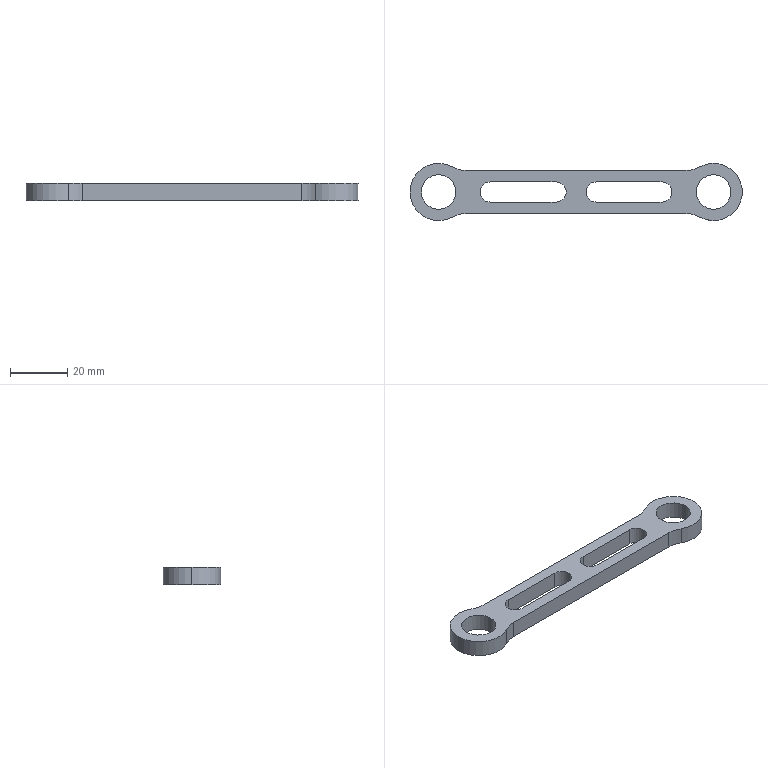Part | SolidWorks | features Extrusion 1, Fillet 1 | 1 solid | 25 faces | box 116 x 20 x 6 mm | volume 7064 mm3 | cylinder 17 | plane 8 | commonest cylinder face diameters 20 x7 7 x6 12 x4
STEP:
#1=CARTESIAN_POINT('',(55.,3.5,6.));
#2=VERTEX_POINT('',#1);
#3=CARTESIAN_POINT('',(51.5,0.,6.));
#4=VERTEX_POINT('',#3);
#5=CARTESIAN_POINT('',(55.,0.,6.));
#6=DIRECTION('',(0.,0.,1.));
#7=DIRECTION('',(1.,0.,0.));
#8=AXIS2_PLACEMENT_3D('',#5,#6,#7);
#9=CIRCLE('',#8,3.5);
#10=EDGE_CURVE('',#2,#4,#9,.T.);
#11=ORIENTED_EDGE('',*,*,#10,.T.);
#12=CARTESIAN_POINT('',(51.5,0.,0.));
#13=VERTEX_POINT('',#12);
#14=CARTESIAN_POINT('',(51.5,0.,6.));
#15=DIRECTION('',(0.,0.,-1.));
#16=VECTOR('',#15,1000.);
#17=LINE('',#14,#16);
#18=EDGE_CURVE('',#4,#13,#17,.T.);
#19=ORIENTED_EDGE('',*,*,#18,.T.);
#20=CARTESIAN_POINT('',(55.,3.5,0.));
#21=VERTEX_POINT('',#20);
#22=CARTESIAN_POINT('',(55.,0.,0.));
#23=DIRECTION('',(0.,0.,1.));
#24=DIRECTION('',(1.,0.,0.));
#25=AXIS2_PLACEMENT_3D('',#22,#23,#24);
#26=CIRCLE('',#25,3.5);
#27=EDGE_CURVE('',#21,#13,#26,.T.);
#28=ORIENTED_EDGE('',*,*,#27,.F.);
#29=CARTESIAN_POINT('',(55.,3.5,6.));
#30=DIRECTION('',(0.,0.,-1.));
#31=VECTOR('',#30,1000.);
#32=LINE('',#29,#31);
#33=EDGE_CURVE('',#2,#21,#32,.T.);
#34=ORIENTED_EDGE('',*,*,#33,.F.);
#35=EDGE_LOOP('',(#11,#19,#28,#34));
#36=FACE_OUTER_BOUND('',#35,.T.);
#37=CARTESIAN_POINT('',(55.,0.,6.));
#38=DIRECTION('',(0.,0.,-1.));
#39=DIRECTION('',(-1.,0.,0.));
#40=AXIS2_PLACEMENT_3D('',#37,#38,#39);
#41=CYLINDRICAL_SURFACE('',#40,3.5);
#42=ADVANCED_FACE('',(#36),#41,.F.);
#43=CARTESIAN_POINT('',(18.,3.5,6.));
#44=VERTEX_POINT('',#43);
#45=CARTESIAN_POINT('',(14.5,0.,6.));
#46=VERTEX_POINT('',#45);
#47=CARTESIAN_POINT('',(18.,0.,6.));
#48=DIRECTION('',(0.,0.,1.));
#49=DIRECTION('',(1.,0.,0.));
#50=AXIS2_PLACEMENT_3D('',#47,#48,#49);
#51=CIRCLE('',#50,3.5);
#52=EDGE_CURVE('',#44,#46,#51,.T.);
#53=ORIENTED_EDGE('',*,*,#52,.T.);
#54=CARTESIAN_POINT('',(14.5,0.,0.));
#55=VERTEX_POINT('',#54);
#56=CARTESIAN_POINT('',(14.5,0.,6.));
#57=DIRECTION('',(0.,0.,-1.));
#58=VECTOR('',#57,1000.);
#59=LINE('',#56,#58);
#60=EDGE_CURVE('',#46,#55,#59,.T.);
#61=ORIENTED_EDGE('',*,*,#60,.T.);
#62=CARTESIAN_POINT('',(18.,3.5,0.));
#63=VERTEX_POINT('',#62);
#64=CARTESIAN_POINT('',(18.,0.,0.));
#65=DIRECTION('',(0.,0.,1.));
#66=DIRECTION('',(1.,0.,0.));
#67=AXIS2_PLACEMENT_3D('',#64,#65,#66);
#68=CIRCLE('',#67,3.5);
#69=EDGE_CURVE('',#63,#55,#68,.T.);
#70=ORIENTED_EDGE('',*,*,#69,.F.);
#71=CARTESIAN_POINT('',(18.,3.5,6.));
#72=DIRECTION('',(0.,0.,-1.));
#73=VECTOR('',#72,1000.);
#74=LINE('',#71,#73);
#75=EDGE_CURVE('',#44,#63,#74,.T.);
#76=ORIENTED_EDGE('',*,*,#75,.F.);
#77=EDGE_LOOP('',(#53,#61,#70,#76));
#78=FACE_OUTER_BOUND('',#77,.T.);
#79=CARTESIAN_POINT('',(18.,0.,6.));
#80=DIRECTION('',(0.,0.,-1.));
#81=DIRECTION('',(-1.,0.,0.));
#82=AXIS2_PLACEMENT_3D('',#79,#80,#81);
#83=CYLINDRICAL_SURFACE('',#82,3.5);
#84=ADVANCED_FACE('',(#78),#83,.F.);
#85=CARTESIAN_POINT('',(90.,0.,6.));
#86=VERTEX_POINT('',#85);
#87=CARTESIAN_POINT('',(102.,0.,6.));
#88=VERTEX_POINT('',#87);
#89=CARTESIAN_POINT('',(96.,0.,6.));
#90=DIRECTION('',(0.,0.,1.));
#91=DIRECTION('',(1.,0.,0.));
#92=AXIS2_PLACEMENT_3D('',#89,#90,#91);
#93=CIRCLE('',#92,6.);
#94=EDGE_CURVE('',#86,#88,#93,.T.);
#95=ORIENTED_EDGE('',*,*,#94,.T.);
#96=CARTESIAN_POINT('',(102.,0.,0.));
#97=VERTEX_POINT('',#96);
#98=CARTESIAN_POINT('',(102.,0.,6.));
#99=DIRECTION('',(0.,0.,-1.));
#100=VECTOR('',#99,1000.);
#101=LINE('',#98,#100);
#102=EDGE_CURVE('',#88,#97,#101,.T.);
#103=ORIENTED_EDGE('',*,*,#102,.T.);
#104=CARTESIAN_POINT('',(90.,0.,0.));
#105=VERTEX_POINT('',#104);
#106=CARTESIAN_POINT('',(96.,0.,0.));
#107=DIRECTION('',(0.,0.,1.));
#108=DIRECTION('',(1.,0.,0.));
#109=AXIS2_PLACEMENT_3D('',#106,#107,#108);
#110=CIRCLE('',#109,6.);
#111=EDGE_CURVE('',#105,#97,#110,.T.);
#112=ORIENTED_EDGE('',*,*,#111,.F.);
#113=CARTESIAN_POINT('',(90.,0.,6.));
#114=DIRECTION('',(0.,0.,-1.));
#115=VECTOR('',#114,1000.);
#116=LINE('',#113,#115);
#117=EDGE_CURVE('',#86,#105,#116,.T.);
#118=ORIENTED_EDGE('',*,*,#117,.F.);
#119=EDGE_LOOP('',(#95,#103,#112,#118));
#120=FACE_OUTER_BOUND('',#119,.T.);
#121=CARTESIAN_POINT('',(96.,0.,6.));
#122=DIRECTION('',(0.,0.,-1.));
#123=DIRECTION('',(-1.,0.,0.));
#124=AXIS2_PLACEMENT_3D('',#121,#122,#123);
#125=CYLINDRICAL_SURFACE('',#124,6.);
#126=ADVANCED_FACE('',(#120),#125,.F.);
#127=CARTESIAN_POINT('',(-6.,0.,6.));
#128=VERTEX_POINT('',#127);
#129=CARTESIAN_POINT('',(6.,0.,6.));
#130=VERTEX_POINT('',#129);
#131=CARTESIAN_POINT('',(0.,0.,6.));
#132=DIRECTION('',(0.,0.,1.));
#133=DIRECTION('',(1.,0.,0.));
#134=AXIS2_PLACEMENT_3D('',#131,#132,#133);
#135=CIRCLE('',#134,6.);
#136=EDGE_CURVE('',#128,#130,#135,.T.);
#137=ORIENTED_EDGE('',*,*,#136,.T.);
#138=CARTESIAN_POINT('',(6.,0.,0.));
#139=VERTEX_POINT('',#138);
#140=CARTESIAN_POINT('',(6.,0.,6.));
#141=DIRECTION('',(0.,0.,-1.));
#142=VECTOR('',#141,1000.);
#143=LINE('',#140,#142);
#144=EDGE_CURVE('',#130,#139,#143,.T.);
#145=ORIENTED_EDGE('',*,*,#144,.T.);
#146=CARTESIAN_POINT('',(-6.,0.,0.));
#147=VERTEX_POINT('',#146);
#148=CARTESIAN_POINT('',(0.,0.,0.));
#149=DIRECTION('',(0.,0.,1.));
#150=DIRECTION('',(1.,0.,0.));
#151=AXIS2_PLACEMENT_3D('',#148,#149,#150);
#152=CIRCLE('',#151,6.);
#153=EDGE_CURVE('',#147,#139,#152,.T.);
#154=ORIENTED_EDGE('',*,*,#153,.F.);
#155=CARTESIAN_POINT('',(-6.,0.,6.));
#156=DIRECTION('',(0.,0.,-1.));
#157=VECTOR('',#156,1000.);
#158=LINE('',#155,#157);
#159=EDGE_CURVE('',#128,#147,#158,.T.);
#160=ORIENTED_EDGE('',*,*,#159,.F.);
#161=EDGE_LOOP('',(#137,#145,#154,#160));
#162=FACE_OUTER_BOUND('',#161,.T.);
#163=CARTESIAN_POINT('',(0.,0.,6.));
#164=DIRECTION('',(0.,0.,-1.));
#165=DIRECTION('',(-1.,0.,0.));
#166=AXIS2_PLACEMENT_3D('',#163,#164,#165);
#167=CYLINDRICAL_SURFACE('',#166,6.);
#168=ADVANCED_FACE('',(#162),#167,.F.);
#169=CARTESIAN_POINT('',(-10.,0.,6.));
#170=VERTEX_POINT('',#169);
#171=CARTESIAN_POINT('',(4.841,-8.75,6.));
#172=VERTEX_POINT('',#171);
#173=CARTESIAN_POINT('',(0.,0.,6.));
#174=DIRECTION('',(0.,0.,1.));
#175=DIRECTION('',(1.,0.,0.));
#176=AXIS2_PLACEMENT_3D('',#173,#174,#175);
#177=CIRCLE('',#176,10.);
#178=EDGE_CURVE('',#170,#172,#177,.T.);
#179=ORIENTED_EDGE('',*,*,#178,.F.);
#180=CARTESIAN_POINT('',(-10.,0.,0.));
#181=VERTEX_POINT('',#180);
#182=CARTESIAN_POINT('',(-10.,0.,6.));
#183=DIRECTION('',(0.,0.,-1.));
#184=VECTOR('',#183,1000.);
#185=LINE('',#182,#184);
#186=EDGE_CURVE('',#170,#181,#185,.T.);
#187=ORIENTED_EDGE('',*,*,#186,.T.);
#188=CARTESIAN_POINT('',(4.841,-8.75,0.));
#189=VERTEX_POINT('',#188);
#190=CARTESIAN_POINT('',(0.,0.,0.));
#191=DIRECTION('',(0.,0.,1.));
#192=DIRECTION('',(1.,0.,0.));
#193=AXIS2_PLACEMENT_3D('',#190,#191,#192);
#194=CIRCLE('',#193,10.);
#195=EDGE_CURVE('',#181,#189,#194,.T.);
#196=ORIENTED_EDGE('',*,*,#195,.T.);
#197=CARTESIAN_POINT('',(4.841,-8.75,6.));
#198=DIRECTION('',(0.,0.,1.));
#199=VECTOR('',#198,1000.);
#200=LINE('',#197,#199);
#201=EDGE_CURVE('',#189,#172,#200,.T.);
#202=ORIENTED_EDGE('',*,*,#201,.T.);
#203=EDGE_LOOP('',(#179,#187,#196,#202));
#204=FACE_OUTER_BOUND('',#203,.T.);
#205=CARTESIAN_POINT('',(0.,0.,6.));
#206=DIRECTION('',(0.,0.,-1.));
#207=DIRECTION('',(-1.,0.,0.));
#208=AXIS2_PLACEMENT_3D('',#205,#206,#207);
#209=CYLINDRICAL_SURFACE('',#208,10.);
#210=ADVANCED_FACE('',(#204),#209,.T.);
#211=ORIENTED_EDGE('',*,*,#136,.F.);
#212=CARTESIAN_POINT('',(0.,0.,6.));
#213=DIRECTION('',(0.,0.,1.));
#214=DIRECTION('',(1.,0.,0.));
#215=AXIS2_PLACEMENT_3D('',#212,#213,#214);
#216=CIRCLE('',#215,6.);
#217=EDGE_CURVE('',#130,#128,#216,.T.);
#218=ORIENTED_EDGE('',*,*,#217,.F.);
#219=EDGE_LOOP('',(#211,#218));
#220=FACE_BOUND('',#219,.T.);
#221=CARTESIAN_POINT('',(86.318,7.5,6.));
#222=VERTEX_POINT('',#221);
#223=CARTESIAN_POINT('',(9.682,7.5,6.));
#224=VERTEX_POINT('',#223);
#225=CARTESIAN_POINT('',(6.614,7.5,6.));
#226=DIRECTION('',(-1.,0.,0.));
#227=VECTOR('',#226,1000.);
#228=LINE('',#225,#227);
#229=EDGE_CURVE('',#222,#224,#228,.T.);
#230=ORIENTED_EDGE('',*,*,#229,.T.);
#231=CARTESIAN_POINT('',(4.841,8.75,6.));
#232=VERTEX_POINT('',#231);
#233=CARTESIAN_POINT('',(9.682,17.5,6.));
#234=DIRECTION('',(0.,0.,-1.));
#235=DIRECTION('',(1.,0.,0.));
#236=AXIS2_PLACEMENT_3D('',#233,#234,#235);
#237=CIRCLE('',#236,10.);
#238=EDGE_CURVE('',#224,#232,#237,.T.);
#239=ORIENTED_EDGE('',*,*,#238,.T.);
#240=CARTESIAN_POINT('',(0.,0.,6.));
#241=DIRECTION('',(0.,0.,1.));
#242=DIRECTION('',(1.,0.,0.));
#243=AXIS2_PLACEMENT_3D('',#240,#241,#242);
#244=CIRCLE('',#243,10.);
#245=EDGE_CURVE('',#232,#170,#244,.T.);
#246=ORIENTED_EDGE('',*,*,#245,.T.);
#247=ORIENTED_EDGE('',*,*,#178,.T.);
#248=CARTESIAN_POINT('',(9.682,-7.5,6.));
#249=VERTEX_POINT('',#248);
#250=CARTESIAN_POINT('',(9.682,-17.5,6.));
#251=DIRECTION('',(0.,0.,-1.));
#252=DIRECTION('',(1.,0.,0.));
#253=AXIS2_PLACEMENT_3D('',#250,#251,#252);
#254=CIRCLE('',#253,10.);
#255=EDGE_CURVE('',#172,#249,#254,.T.);
#256=ORIENTED_EDGE('',*,*,#255,.T.);
#257=CARTESIAN_POINT('',(86.318,-7.5,6.));
#258=VERTEX_POINT('',#257);
#259=CARTESIAN_POINT('',(6.614,-7.5,6.));
#260=DIRECTION('',(1.,0.,0.));
#261=VECTOR('',#260,1000.);
#262=LINE('',#259,#261);
#263=EDGE_CURVE('',#249,#258,#262,.T.);
#264=ORIENTED_EDGE('',*,*,#263,.T.);
#265=CARTESIAN_POINT('',(91.159,-8.75,6.));
#266=VERTEX_POINT('',#265);
#267=CARTESIAN_POINT('',(86.318,-17.5,6.));
#268=DIRECTION('',(0.,0.,-1.));
#269=DIRECTION('',(1.,0.,0.));
#270=AXIS2_PLACEMENT_3D('',#267,#268,#269);
#271=CIRCLE('',#270,10.);
#272=EDGE_CURVE('',#258,#266,#271,.T.);
#273=ORIENTED_EDGE('',*,*,#272,.T.);
#274=CARTESIAN_POINT('',(91.159,8.75,6.));
#275=VERTEX_POINT('',#274);
#276=CARTESIAN_POINT('',(96.,0.,6.));
#277=DIRECTION('',(0.,0.,1.));
#278=DIRECTION('',(1.,0.,0.));
#279=AXIS2_PLACEMENT_3D('',#276,#277,#278);
#280=CIRCLE('',#279,10.);
#281=EDGE_CURVE('',#266,#275,#280,.T.);
#282=ORIENTED_EDGE('',*,*,#281,.T.);
#283=CARTESIAN_POINT('',(86.318,17.5,6.));
#284=DIRECTION('',(0.,0.,-1.));
#285=DIRECTION('',(1.,0.,0.));
#286=AXIS2_PLACEMENT_3D('',#283,#284,#285);
#287=CIRCLE('',#286,10.);
#288=EDGE_CURVE('',#275,#222,#287,.T.);
#289=ORIENTED_EDGE('',*,*,#288,.T.);
#290=EDGE_LOOP('',(#230,#239,#246,#247,#256,#264,#273,#282,#289));
#291=FACE_OUTER_BOUND('',#290,.T.);
#292=ORIENTED_EDGE('',*,*,#94,.F.);
#293=CARTESIAN_POINT('',(96.,0.,6.));
#294=DIRECTION('',(0.,0.,1.));
#295=DIRECTION('',(1.,0.,0.));
#296=AXIS2_PLACEMENT_3D('',#293,#294,#295);
#297=CIRCLE('',#296,6.);
#298=EDGE_CURVE('',#88,#86,#297,.T.);
#299=ORIENTED_EDGE('',*,*,#298,.F.);
#300=EDGE_LOOP('',(#292,#299));
#301=FACE_BOUND('',#300,.T.);
#302=CARTESIAN_POINT('',(18.,-3.5,6.));
#303=VERTEX_POINT('',#302);
#304=CARTESIAN_POINT('',(41.,-3.5,6.));
#305=VERTEX_POINT('',#304);
#306=CARTESIAN_POINT('',(18.,-3.5,6.));
#307=DIRECTION('',(1.,0.,0.));
#308=VECTOR('',#307,1000.);
#309=LINE('',#306,#308);
#310=EDGE_CURVE('',#303,#305,#309,.T.);
#311=ORIENTED_EDGE('',*,*,#310,.F.);
#312=CARTESIAN_POINT('',(18.,0.,6.));
#313=DIRECTION('',(0.,0.,1.));
#314=DIRECTION('',(1.,0.,0.));
#315=AXIS2_PLACEMENT_3D('',#312,#313,#314);
#316=CIRCLE('',#315,3.5);
#317=EDGE_CURVE('',#46,#303,#316,.T.);
#318=ORIENTED_EDGE('',*,*,#317,.F.);
#319=ORIENTED_EDGE('',*,*,#52,.F.);
#320=CARTESIAN_POINT('',(41.,3.5,6.));
#321=VERTEX_POINT('',#320);
#322=CARTESIAN_POINT('',(18.,3.5,6.));
#323=DIRECTION('',(-1.,0.,0.));
#324=VECTOR('',#323,1000.);
#325=LINE('',#322,#324);
#326=EDGE_CURVE('',#321,#44,#325,.T.);
#327=ORIENTED_EDGE('',*,*,#326,.F.);
#328=CARTESIAN_POINT('',(41.,0.,6.));
#329=DIRECTION('',(0.,0.,1.));
#330=DIRECTION('',(1.,0.,0.));
#331=AXIS2_PLACEMENT_3D('',#328,#329,#330);
#332=CIRCLE('',#331,3.5);
#333=EDGE_CURVE('',#305,#321,#332,.T.);
#334=ORIENTED_EDGE('',*,*,#333,.F.);
#335=EDGE_LOOP('',(#311,#318,#319,#327,#334));
#336=FACE_BOUND('',#335,.T.);
#337=CARTESIAN_POINT('',(78.,3.5,6.));
#338=VERTEX_POINT('',#337);
#339=CARTESIAN_POINT('',(78.,3.5,6.));
#340=DIRECTION('',(-1.,0.,0.));
#341=VECTOR('',#340,1000.);
#342=LINE('',#339,#341);
#343=EDGE_CURVE('',#338,#2,#342,.T.);
#344=ORIENTED_EDGE('',*,*,#343,.F.);
#345=CARTESIAN_POINT('',(78.,-3.5,6.));
#346=VERTEX_POINT('',#345);
#347=CARTESIAN_POINT('',(78.,0.,6.));
#348=DIRECTION('',(0.,0.,1.));
#349=DIRECTION('',(1.,0.,0.));
#350=AXIS2_PLACEMENT_3D('',#347,#348,#349);
#351=CIRCLE('',#350,3.5);
#352=EDGE_CURVE('',#346,#338,#351,.T.);
#353=ORIENTED_EDGE('',*,*,#352,.F.);
#354=CARTESIAN_POINT('',(55.,-3.5,6.));
#355=VERTEX_POINT('',#354);
#356=CARTESIAN_POINT('',(78.,-3.5,6.));
#357=DIRECTION('',(1.,0.,0.));
#358=VECTOR('',#357,1000.);
#359=LINE('',#356,#358);
#360=EDGE_CURVE('',#355,#346,#359,.T.);
#361=ORIENTED_EDGE('',*,*,#360,.F.);
#362=CARTESIAN_POINT('',(55.,0.,6.));
#363=DIRECTION('',(0.,0.,1.));
#364=DIRECTION('',(1.,0.,0.));
#365=AXIS2_PLACEMENT_3D('',#362,#363,#364);
#366=CIRCLE('',#365,3.5);
#367=EDGE_CURVE('',#4,#355,#366,.T.);
#368=ORIENTED_EDGE('',*,*,#367,.F.);
#369=ORIENTED_EDGE('',*,*,#10,.F.);
#370=EDGE_LOOP('',(#344,#353,#361,#368,#369));
#371=FACE_BOUND('',#370,.T.);
#372=CARTESIAN_POINT('',(0.,0.,6.));
#373=DIRECTION('',(0.,0.,1.));
#374=DIRECTION('',(1.,0.,0.));
#375=AXIS2_PLACEMENT_3D('',#372,#373,#374);
#376=PLANE('',#375);
#377=ADVANCED_FACE('',(#220,#291,#301,#336,#371),#376,.T.);
#378=ORIENTED_EDGE('',*,*,#69,.T.);
#379=CARTESIAN_POINT('',(18.,-3.5,0.));
#380=VERTEX_POINT('',#379);
#381=CARTESIAN_POINT('',(18.,0.,0.));
#382=DIRECTION('',(0.,0.,1.));
#383=DIRECTION('',(1.,0.,0.));
#384=AXIS2_PLACEMENT_3D('',#381,#382,#383);
#385=CIRCLE('',#384,3.5);
#386=EDGE_CURVE('',#55,#380,#385,.T.);
#387=ORIENTED_EDGE('',*,*,#386,.T.);
#388=CARTESIAN_POINT('',(41.,-3.5,0.));
#389=VERTEX_POINT('',#388);
#390=CARTESIAN_POINT('',(18.,-3.5,0.));
#391=DIRECTION('',(1.,0.,0.));
#392=VECTOR('',#391,1000.);
#393=LINE('',#390,#392);
#394=EDGE_CURVE('',#380,#389,#393,.T.);
#395=ORIENTED_EDGE('',*,*,#394,.T.);
#396=CARTESIAN_POINT('',(41.,3.5,0.));
#397=VERTEX_POINT('',#396);
#398=CARTESIAN_POINT('',(41.,0.,0.));
#399=DIRECTION('',(0.,0.,1.));
#400=DIRECTION('',(1.,0.,0.));
#401=AXIS2_PLACEMENT_3D('',#398,#399,#400);
#402=CIRCLE('',#401,3.5);
#403=EDGE_CURVE('',#389,#397,#402,.T.);
#404=ORIENTED_EDGE('',*,*,#403,.T.);
#405=CARTESIAN_POINT('',(18.,3.5,0.));
#406=DIRECTION('',(-1.,0.,0.));
#407=VECTOR('',#406,1000.);
#408=LINE('',#405,#407);
#409=EDGE_CURVE('',#397,#63,#408,.T.);
#410=ORIENTED_EDGE('',*,*,#409,.T.);
#411=EDGE_LOOP('',(#378,#387,#395,#404,#410));
#412=FACE_BOUND('',#411,.T.);
#413=CARTESIAN_POINT('',(4.841,8.75,0.));
#414=VERTEX_POINT('',#413);
#415=CARTESIAN_POINT('',(0.,0.,0.));
#416=DIRECTION('',(0.,0.,1.));
#417=DIRECTION('',(1.,0.,0.));
#418=AXIS2_PLACEMENT_3D('',#415,#416,#417);
#419=CIRCLE('',#418,10.);
#420=EDGE_CURVE('',#414,#181,#419,.T.);
#421=ORIENTED_EDGE('',*,*,#420,.F.);
#422=CARTESIAN_POINT('',(9.682,7.5,0.));
#423=VERTEX_POINT('',#422);
#424=CARTESIAN_POINT('',(9.682,17.5,0.));
#425=DIRECTION('',(0.,0.,1.));
#426=DIRECTION('',(1.,0.,0.));
#427=AXIS2_PLACEMENT_3D('',#424,#425,#426);
#428=CIRCLE('',#427,10.);
#429=EDGE_CURVE('',#414,#423,#428,.T.);
#430=ORIENTED_EDGE('',*,*,#429,.T.);
#431=CARTESIAN_POINT('',(86.318,7.5,0.));
#432=VERTEX_POINT('',#431);
#433=CARTESIAN_POINT('',(6.614,7.5,0.));
#434=DIRECTION('',(-1.,0.,0.));
#435=VECTOR('',#434,1000.);
#436=LINE('',#433,#435);
#437=EDGE_CURVE('',#432,#423,#436,.T.);
#438=ORIENTED_EDGE('',*,*,#437,.F.);
#439=CARTESIAN_POINT('',(91.159,8.75,0.));
#440=VERTEX_POINT('',#439);
#441=CARTESIAN_POINT('',(86.318,17.5,0.));
#442=DIRECTION('',(0.,0.,1.));
#443=DIRECTION('',(1.,0.,0.));
#444=AXIS2_PLACEMENT_3D('',#441,#442,#443);
#445=CIRCLE('',#444,10.);
#446=EDGE_CURVE('',#432,#440,#445,.T.);
#447=ORIENTED_EDGE('',*,*,#446,.T.);
#448=CARTESIAN_POINT('',(91.159,-8.75,0.));
#449=VERTEX_POINT('',#448);
#450=CARTESIAN_POINT('',(96.,0.,0.));
#451=DIRECTION('',(0.,0.,1.));
#452=DIRECTION('',(1.,0.,0.));
#453=AXIS2_PLACEMENT_3D('',#450,#451,#452);
#454=CIRCLE('',#453,10.);
#455=EDGE_CURVE('',#449,#440,#454,.T.);
#456=ORIENTED_EDGE('',*,*,#455,.F.);
#457=CARTESIAN_POINT('',(86.318,-7.5,0.));
#458=VERTEX_POINT('',#457);
#459=CARTESIAN_POINT('',(86.318,-17.5,0.));
#460=DIRECTION('',(0.,0.,1.));
#461=DIRECTION('',(1.,0.,0.));
#462=AXIS2_PLACEMENT_3D('',#459,#460,#461);
#463=CIRCLE('',#462,10.);
#464=EDGE_CURVE('',#449,#458,#463,.T.);
#465=ORIENTED_EDGE('',*,*,#464,.T.);
#466=CARTESIAN_POINT('',(9.682,-7.5,0.));
#467=VERTEX_POINT('',#466);
#468=CARTESIAN_POINT('',(6.614,-7.5,0.));
#469=DIRECTION('',(1.,0.,0.));
#470=VECTOR('',#469,1000.);
#471=LINE('',#468,#470);
#472=EDGE_CURVE('',#467,#458,#471,.T.);
#473=ORIENTED_EDGE('',*,*,#472,.F.);
#474=CARTESIAN_POINT('',(9.682,-17.5,0.));
#475=DIRECTION('',(0.,0.,1.));
#476=DIRECTION('',(1.,0.,0.));
#477=AXIS2_PLACEMENT_3D('',#474,#475,#476);
#478=CIRCLE('',#477,10.);
#479=EDGE_CURVE('',#467,#189,#478,.T.);
#480=ORIENTED_EDGE('',*,*,#479,.T.);
#481=ORIENTED_EDGE('',*,*,#195,.F.);
#482=EDGE_LOOP('',(#421,#430,#438,#447,#456,#465,#473,#480,#481));
#483=FACE_OUTER_BOUND('',#482,.T.);
#484=ORIENTED_EDGE('',*,*,#153,.T.);
#485=CARTESIAN_POINT('',(0.,0.,0.));
#486=DIRECTION('',(0.,0.,1.));
#487=DIRECTION('',(1.,0.,0.));
#488=AXIS2_PLACEMENT_3D('',#485,#486,#487);
#489=CIRCLE('',#488,6.);
#490=EDGE_CURVE('',#139,#147,#489,.T.);
#491=ORIENTED_EDGE('',*,*,#490,.T.);
#492=EDGE_LOOP('',(#484,#491));
#493=FACE_BOUND('',#492,.T.);
#494=ORIENTED_EDGE('',*,*,#111,.T.);
#495=CARTESIAN_POINT('',(96.,0.,0.));
#496=DIRECTION('',(0.,0.,1.));
#497=DIRECTION('',(1.,0.,0.));
#498=AXIS2_PLACEMENT_3D('',#495,#496,#497);
#499=CIRCLE('',#498,6.);
#500=EDGE_CURVE('',#97,#105,#499,.T.);
#501=ORIENTED_EDGE('',*,*,#500,.T.);
#502=EDGE_LOOP('',(#494,#501));
#503=FACE_BOUND('',#502,.T.);
#504=CARTESIAN_POINT('',(78.,-3.5,0.));
#505=VERTEX_POINT('',#504);
#506=CARTESIAN_POINT('',(78.,3.5,0.));
#507=VERTEX_POINT('',#506);
#508=CARTESIAN_POINT('',(78.,0.,0.));
#509=DIRECTION('',(0.,0.,1.));
#510=DIRECTION('',(1.,0.,0.));
#511=AXIS2_PLACEMENT_3D('',#508,#509,#510);
#512=CIRCLE('',#511,3.5);
#513=EDGE_CURVE('',#505,#507,#512,.T.);
#514=ORIENTED_EDGE('',*,*,#513,.T.);
#515=CARTESIAN_POINT('',(78.,3.5,0.));
#516=DIRECTION('',(-1.,0.,0.));
#517=VECTOR('',#516,1000.);
#518=LINE('',#515,#517);
#519=EDGE_CURVE('',#507,#21,#518,.T.);
#520=ORIENTED_EDGE('',*,*,#519,.T.);
#521=ORIENTED_EDGE('',*,*,#27,.T.);
#522=CARTESIAN_POINT('',(55.,-3.5,0.));
#523=VERTEX_POINT('',#522);
#524=CARTESIAN_POINT('',(55.,0.,0.));
#525=DIRECTION('',(0.,0.,1.));
#526=DIRECTION('',(1.,0.,0.));
#527=AXIS2_PLACEMENT_3D('',#524,#525,#526);
#528=CIRCLE('',#527,3.5);
#529=EDGE_CURVE('',#13,#523,#528,.T.);
#530=ORIENTED_EDGE('',*,*,#529,.T.);
#531=CARTESIAN_POINT('',(78.,-3.5,0.));
#532=DIRECTION('',(1.,0.,0.));
#533=VECTOR('',#532,1000.);
#534=LINE('',#531,#533);
#535=EDGE_CURVE('',#523,#505,#534,.T.);
#536=ORIENTED_EDGE('',*,*,#535,.T.);
#537=EDGE_LOOP('',(#514,#520,#521,#530,#536));
#538=FACE_BOUND('',#537,.T.);
#539=CARTESIAN_POINT('',(0.,0.,0.));
#540=DIRECTION('',(0.,0.,1.));
#541=DIRECTION('',(1.,0.,0.));
#542=AXIS2_PLACEMENT_3D('',#539,#540,#541);
#543=PLANE('',#542);
#544=ADVANCED_FACE('',(#412,#483,#493,#503,#538),#543,.F.);
#545=ORIENTED_EDGE('',*,*,#186,.F.);
#546=ORIENTED_EDGE('',*,*,#245,.F.);
#547=CARTESIAN_POINT('',(4.841,8.75,6.));
#548=DIRECTION('',(0.,0.,-1.));
#549=VECTOR('',#548,1000.);
#550=LINE('',#547,#549);
#551=EDGE_CURVE('',#232,#414,#550,.T.);
#552=ORIENTED_EDGE('',*,*,#551,.T.);
#553=ORIENTED_EDGE('',*,*,#420,.T.);
#554=EDGE_LOOP('',(#545,#546,#552,#553));
#555=FACE_OUTER_BOUND('',#554,.T.);
#556=CARTESIAN_POINT('',(0.,0.,6.));
#557=DIRECTION('',(0.,0.,-1.));
#558=DIRECTION('',(-1.,0.,0.));
#559=AXIS2_PLACEMENT_3D('',#556,#557,#558);
#560=CYLINDRICAL_SURFACE('',#559,10.);
#561=ADVANCED_FACE('',(#555),#560,.T.);
#562=ORIENTED_EDGE('',*,*,#263,.F.);
#563=CARTESIAN_POINT('',(9.682,-7.5,0.));
#564=DIRECTION('',(0.,0.,-1.));
#565=VECTOR('',#564,1000.);
#566=LINE('',#563,#565);
#567=EDGE_CURVE('',#249,#467,#566,.T.);
#568=ORIENTED_EDGE('',*,*,#567,.T.);
#569=ORIENTED_EDGE('',*,*,#472,.T.);
#570=CARTESIAN_POINT('',(86.318,-7.5,6.));
#571=DIRECTION('',(0.,0.,1.));
#572=VECTOR('',#571,1000.);
#573=LINE('',#570,#572);
#574=EDGE_CURVE('',#458,#258,#573,.T.);
#575=ORIENTED_EDGE('',*,*,#574,.T.);
#576=EDGE_LOOP('',(#562,#568,#569,#575));
#577=FACE_OUTER_BOUND('',#576,.T.);
#578=CARTESIAN_POINT('',(6.614,-7.5,6.));
#579=DIRECTION('',(0.,1.,0.));
#580=DIRECTION('',(0.,0.,1.));
#581=AXIS2_PLACEMENT_3D('',#578,#579,#580);
#582=PLANE('',#581);
#583=ADVANCED_FACE('',(#577),#582,.F.);
#584=ORIENTED_EDGE('',*,*,#281,.F.);
#585=CARTESIAN_POINT('',(91.159,-8.75,6.));
#586=DIRECTION('',(0.,0.,-1.));
#587=VECTOR('',#586,1000.);
#588=LINE('',#585,#587);
#589=EDGE_CURVE('',#266,#449,#588,.T.);
#590=ORIENTED_EDGE('',*,*,#589,.T.);
#591=ORIENTED_EDGE('',*,*,#455,.T.);
#592=CARTESIAN_POINT('',(91.159,8.75,6.));
#593=DIRECTION('',(0.,0.,1.));
#594=VECTOR('',#593,1000.);
#595=LINE('',#592,#594);
#596=EDGE_CURVE('',#440,#275,#595,.T.);
#597=ORIENTED_EDGE('',*,*,#596,.T.);
#598=EDGE_LOOP('',(#584,#590,#591,#597));
#599=FACE_OUTER_BOUND('',#598,.T.);
#600=CARTESIAN_POINT('',(96.,0.,6.));
#601=DIRECTION('',(0.,0.,-1.));
#602=DIRECTION('',(-1.,0.,0.));
#603=AXIS2_PLACEMENT_3D('',#600,#601,#602);
#604=CYLINDRICAL_SURFACE('',#603,10.);
#605=ADVANCED_FACE('',(#599),#604,.T.);
#606=ORIENTED_EDGE('',*,*,#229,.F.);
#607=CARTESIAN_POINT('',(86.318,7.5,0.));
#608=DIRECTION('',(0.,0.,-1.));
#609=VECTOR('',#608,1000.);
#610=LINE('',#607,#609);
#611=EDGE_CURVE('',#222,#432,#610,.T.);
#612=ORIENTED_EDGE('',*,*,#611,.T.);
#613=ORIENTED_EDGE('',*,*,#437,.T.);
#614=CARTESIAN_POINT('',(9.682,7.5,6.));
#615=DIRECTION('',(0.,0.,1.));
#616=VECTOR('',#615,1000.);
#617=LINE('',#614,#616);
#618=EDGE_CURVE('',#423,#224,#617,.T.);
#619=ORIENTED_EDGE('',*,*,#618,.T.);
#620=EDGE_LOOP('',(#606,#612,#613,#619));
#621=FACE_OUTER_BOUND('',#620,.T.);
#622=CARTESIAN_POINT('',(6.614,7.5,6.));
#623=DIRECTION('',(0.,-1.,0.));
#624=DIRECTION('',(0.,0.,-1.));
#625=AXIS2_PLACEMENT_3D('',#622,#623,#624);
#626=PLANE('',#625);
#627=ADVANCED_FACE('',(#621),#626,.F.);
#628=ORIENTED_EDGE('',*,*,#144,.F.);
#629=ORIENTED_EDGE('',*,*,#217,.T.);
#630=ORIENTED_EDGE('',*,*,#159,.T.);
#631=ORIENTED_EDGE('',*,*,#490,.F.);
#632=EDGE_LOOP('',(#628,#629,#630,#631));
#633=FACE_OUTER_BOUND('',#632,.T.);
#634=CARTESIAN_POINT('',(0.,0.,6.));
#635=DIRECTION('',(0.,0.,-1.));
#636=DIRECTION('',(-1.,0.,0.));
#637=AXIS2_PLACEMENT_3D('',#634,#635,#636);
#638=CYLINDRICAL_SURFACE('',#637,6.);
#639=ADVANCED_FACE('',(#633),#638,.F.);
#640=ORIENTED_EDGE('',*,*,#102,.F.);
#641=ORIENTED_EDGE('',*,*,#298,.T.);
#642=ORIENTED_EDGE('',*,*,#117,.T.);
#643=ORIENTED_EDGE('',*,*,#500,.F.);
#644=EDGE_LOOP('',(#640,#641,#642,#643));
#645=FACE_OUTER_BOUND('',#644,.T.);
#646=CARTESIAN_POINT('',(96.,0.,6.));
#647=DIRECTION('',(0.,0.,-1.));
#648=DIRECTION('',(-1.,0.,0.));
#649=AXIS2_PLACEMENT_3D('',#646,#647,#648);
#650=CYLINDRICAL_SURFACE('',#649,6.);
#651=ADVANCED_FACE('',(#645),#650,.F.);
#652=ORIENTED_EDGE('',*,*,#60,.F.);
#653=ORIENTED_EDGE('',*,*,#317,.T.);
#654=CARTESIAN_POINT('',(18.,-3.5,6.));
#655=DIRECTION('',(0.,0.,-1.));
#656=VECTOR('',#655,1000.);
#657=LINE('',#654,#656);
#658=EDGE_CURVE('',#303,#380,#657,.T.);
#659=ORIENTED_EDGE('',*,*,#658,.T.);
#660=ORIENTED_EDGE('',*,*,#386,.F.);
#661=EDGE_LOOP('',(#652,#653,#659,#660));
#662=FACE_OUTER_BOUND('',#661,.T.);
#663=CARTESIAN_POINT('',(18.,0.,6.));
#664=DIRECTION('',(0.,0.,-1.));
#665=DIRECTION('',(-1.,0.,0.));
#666=AXIS2_PLACEMENT_3D('',#663,#664,#665);
#667=CYLINDRICAL_SURFACE('',#666,3.5);
#668=ADVANCED_FACE('',(#662),#667,.F.);
#669=ORIENTED_EDGE('',*,*,#394,.F.);
#670=ORIENTED_EDGE('',*,*,#658,.F.);
#671=ORIENTED_EDGE('',*,*,#310,.T.);
#672=CARTESIAN_POINT('',(41.,-3.5,6.));
#673=DIRECTION('',(0.,0.,-1.));
#674=VECTOR('',#673,1000.);
#675=LINE('',#672,#674);
#676=EDGE_CURVE('',#305,#389,#675,.T.);
#677=ORIENTED_EDGE('',*,*,#676,.T.);
#678=EDGE_LOOP('',(#669,#670,#671,#677));
#679=FACE_OUTER_BOUND('',#678,.T.);
#680=CARTESIAN_POINT('',(18.,-3.5,6.));
#681=DIRECTION('',(0.,1.,0.));
#682=DIRECTION('',(0.,0.,1.));
#683=AXIS2_PLACEMENT_3D('',#680,#681,#682);
#684=PLANE('',#683);
#685=ADVANCED_FACE('',(#679),#684,.T.);
#686=ORIENTED_EDGE('',*,*,#403,.F.);
#687=ORIENTED_EDGE('',*,*,#676,.F.);
#688=ORIENTED_EDGE('',*,*,#333,.T.);
#689=CARTESIAN_POINT('',(41.,3.5,6.));
#690=DIRECTION('',(0.,0.,-1.));
#691=VECTOR('',#690,1000.);
#692=LINE('',#689,#691);
#693=EDGE_CURVE('',#321,#397,#692,.T.);
#694=ORIENTED_EDGE('',*,*,#693,.T.);
#695=EDGE_LOOP('',(#686,#687,#688,#694));
#696=FACE_OUTER_BOUND('',#695,.T.);
#697=CARTESIAN_POINT('',(41.,0.,6.));
#698=DIRECTION('',(0.,0.,-1.));
#699=DIRECTION('',(-1.,0.,0.));
#700=AXIS2_PLACEMENT_3D('',#697,#698,#699);
#701=CYLINDRICAL_SURFACE('',#700,3.5);
#702=ADVANCED_FACE('',(#696),#701,.F.);
#703=ORIENTED_EDGE('',*,*,#409,.F.);
#704=ORIENTED_EDGE('',*,*,#693,.F.);
#705=ORIENTED_EDGE('',*,*,#326,.T.);
#706=ORIENTED_EDGE('',*,*,#75,.T.);
#707=EDGE_LOOP('',(#703,#704,#705,#706));
#708=FACE_OUTER_BOUND('',#707,.T.);
#709=CARTESIAN_POINT('',(18.,3.5,6.));
#710=DIRECTION('',(0.,-1.,0.));
#711=DIRECTION('',(0.,0.,-1.));
#712=AXIS2_PLACEMENT_3D('',#709,#710,#711);
#713=PLANE('',#712);
#714=ADVANCED_FACE('',(#708),#713,.T.);
#715=ORIENTED_EDGE('',*,*,#513,.F.);
#716=CARTESIAN_POINT('',(78.,-3.5,6.));
#717=DIRECTION('',(0.,0.,-1.));
#718=VECTOR('',#717,1000.);
#719=LINE('',#716,#718);
#720=EDGE_CURVE('',#346,#505,#719,.T.);
#721=ORIENTED_EDGE('',*,*,#720,.F.);
#722=ORIENTED_EDGE('',*,*,#352,.T.);
#723=CARTESIAN_POINT('',(78.,3.5,6.));
#724=DIRECTION('',(0.,0.,-1.));
#725=VECTOR('',#724,1000.);
#726=LINE('',#723,#725);
#727=EDGE_CURVE('',#338,#507,#726,.T.);
#728=ORIENTED_EDGE('',*,*,#727,.T.);
#729=EDGE_LOOP('',(#715,#721,#722,#728));
#730=FACE_OUTER_BOUND('',#729,.T.);
#731=CARTESIAN_POINT('',(78.,0.,6.));
#732=DIRECTION('',(0.,0.,-1.));
#733=DIRECTION('',(-1.,0.,0.));
#734=AXIS2_PLACEMENT_3D('',#731,#732,#733);
#735=CYLINDRICAL_SURFACE('',#734,3.5);
#736=ADVANCED_FACE('',(#730),#735,.F.);
#737=ORIENTED_EDGE('',*,*,#519,.F.);
#738=ORIENTED_EDGE('',*,*,#727,.F.);
#739=ORIENTED_EDGE('',*,*,#343,.T.);
#740=ORIENTED_EDGE('',*,*,#33,.T.);
#741=EDGE_LOOP('',(#737,#738,#739,#740));
#742=FACE_OUTER_BOUND('',#741,.T.);
#743=CARTESIAN_POINT('',(78.,3.5,6.));
#744=DIRECTION('',(0.,-1.,0.));
#745=DIRECTION('',(0.,0.,-1.));
#746=AXIS2_PLACEMENT_3D('',#743,#744,#745);
#747=PLANE('',#746);
#748=ADVANCED_FACE('',(#742),#747,.T.);
#749=ORIENTED_EDGE('',*,*,#18,.F.);
#750=ORIENTED_EDGE('',*,*,#367,.T.);
#751=CARTESIAN_POINT('',(55.,-3.5,6.));
#752=DIRECTION('',(0.,0.,-1.));
#753=VECTOR('',#752,1000.);
#754=LINE('',#751,#753);
#755=EDGE_CURVE('',#355,#523,#754,.T.);
#756=ORIENTED_EDGE('',*,*,#755,.T.);
#757=ORIENTED_EDGE('',*,*,#529,.F.);
#758=EDGE_LOOP('',(#749,#750,#756,#757));
#759=FACE_OUTER_BOUND('',#758,.T.);
#760=CARTESIAN_POINT('',(55.,0.,6.));
#761=DIRECTION('',(0.,0.,-1.));
#762=DIRECTION('',(-1.,0.,0.));
#763=AXIS2_PLACEMENT_3D('',#760,#761,#762);
#764=CYLINDRICAL_SURFACE('',#763,3.5);
#765=ADVANCED_FACE('',(#759),#764,.F.);
#766=ORIENTED_EDGE('',*,*,#535,.F.);
#767=ORIENTED_EDGE('',*,*,#755,.F.);
#768=ORIENTED_EDGE('',*,*,#360,.T.);
#769=ORIENTED_EDGE('',*,*,#720,.T.);
#770=EDGE_LOOP('',(#766,#767,#768,#769));
#771=FACE_OUTER_BOUND('',#770,.T.);
#772=CARTESIAN_POINT('',(78.,-3.5,6.));
#773=DIRECTION('',(0.,1.,0.));
#774=DIRECTION('',(0.,0.,1.));
#775=AXIS2_PLACEMENT_3D('',#772,#773,#774);
#776=PLANE('',#775);
#777=ADVANCED_FACE('',(#771),#776,.T.);
#778=ORIENTED_EDGE('',*,*,#255,.F.);
#779=ORIENTED_EDGE('',*,*,#201,.F.);
#780=ORIENTED_EDGE('',*,*,#479,.F.);
#781=ORIENTED_EDGE('',*,*,#567,.F.);
#782=EDGE_LOOP('',(#778,#779,#780,#781));
#783=FACE_OUTER_BOUND('',#782,.T.);
#784=CARTESIAN_POINT('',(9.682,-17.5,6.));
#785=DIRECTION('',(0.,0.,-1.));
#786=DIRECTION('',(-1.,0.,0.));
#787=AXIS2_PLACEMENT_3D('',#784,#785,#786);
#788=CYLINDRICAL_SURFACE('',#787,10.);
#789=ADVANCED_FACE('',(#783),#788,.F.);
#790=ORIENTED_EDGE('',*,*,#272,.F.);
#791=ORIENTED_EDGE('',*,*,#574,.F.);
#792=ORIENTED_EDGE('',*,*,#464,.F.);
#793=ORIENTED_EDGE('',*,*,#589,.F.);
#794=EDGE_LOOP('',(#790,#791,#792,#793));
#795=FACE_OUTER_BOUND('',#794,.T.);
#796=CARTESIAN_POINT('',(86.318,-17.5,6.));
#797=DIRECTION('',(0.,0.,-1.));
#798=DIRECTION('',(-1.,0.,0.));
#799=AXIS2_PLACEMENT_3D('',#796,#797,#798);
#800=CYLINDRICAL_SURFACE('',#799,10.);
#801=ADVANCED_FACE('',(#795),#800,.F.);
#802=ORIENTED_EDGE('',*,*,#288,.F.);
#803=ORIENTED_EDGE('',*,*,#596,.F.);
#804=ORIENTED_EDGE('',*,*,#446,.F.);
#805=ORIENTED_EDGE('',*,*,#611,.F.);
#806=EDGE_LOOP('',(#802,#803,#804,#805));
#807=FACE_OUTER_BOUND('',#806,.T.);
#808=CARTESIAN_POINT('',(86.318,17.5,6.));
#809=DIRECTION('',(0.,0.,-1.));
#810=DIRECTION('',(-1.,0.,0.));
#811=AXIS2_PLACEMENT_3D('',#808,#809,#810);
#812=CYLINDRICAL_SURFACE('',#811,10.);
#813=ADVANCED_FACE('',(#807),#812,.F.);
#814=ORIENTED_EDGE('',*,*,#238,.F.);
#815=ORIENTED_EDGE('',*,*,#618,.F.);
#816=ORIENTED_EDGE('',*,*,#429,.F.);
#817=ORIENTED_EDGE('',*,*,#551,.F.);
#818=EDGE_LOOP('',(#814,#815,#816,#817));
#819=FACE_OUTER_BOUND('',#818,.T.);
#820=CARTESIAN_POINT('',(9.682,17.5,6.));
#821=DIRECTION('',(0.,0.,-1.));
#822=DIRECTION('',(-1.,0.,0.));
#823=AXIS2_PLACEMENT_3D('',#820,#821,#822);
#824=CYLINDRICAL_SURFACE('',#823,10.);
#825=ADVANCED_FACE('',(#819),#824,.F.);
#826=CLOSED_SHELL('',(#42,#84,#126,#168,#210,#377,#544,#561,#583,#605,#627,#639,#651,#668,#685,#702,#714,#736,#748,#765,#777,#789,#801,#813,#825));
#827=MANIFOLD_SOLID_BREP('',#826);
#828=CARTESIAN_POINT('',(0.,0.,0.));
#829=DIRECTION('',(0.,0.,1.));
#830=DIRECTION('',(1.,0.,0.));
#831=AXIS2_PLACEMENT_3D('',#828,#829,#830);
#832=(LENGTH_UNIT()NAMED_UNIT(*)SI_UNIT(.MILLI.,.METRE.));
#833=UNCERTAINTY_MEASURE_WITH_UNIT(LENGTH_MEASURE(0.00001),#832,'','');
#834=(NAMED_UNIT(*)PLANE_ANGLE_UNIT()SI_UNIT($,.RADIAN.));
#835=(NAMED_UNIT(*)SI_UNIT($,.STERADIAN.)SOLID_ANGLE_UNIT());
#836=(GEOMETRIC_REPRESENTATION_CONTEXT(3)GLOBAL_UNCERTAINTY_ASSIGNED_CONTEXT((#833))GLOBAL_UNIT_ASSIGNED_CONTEXT((#832,#834,#835))REPRESENTATION_CONTEXT('',''));
#837=ADVANCED_BREP_SHAPE_REPRESENTATION('',(#827,#831),#836);